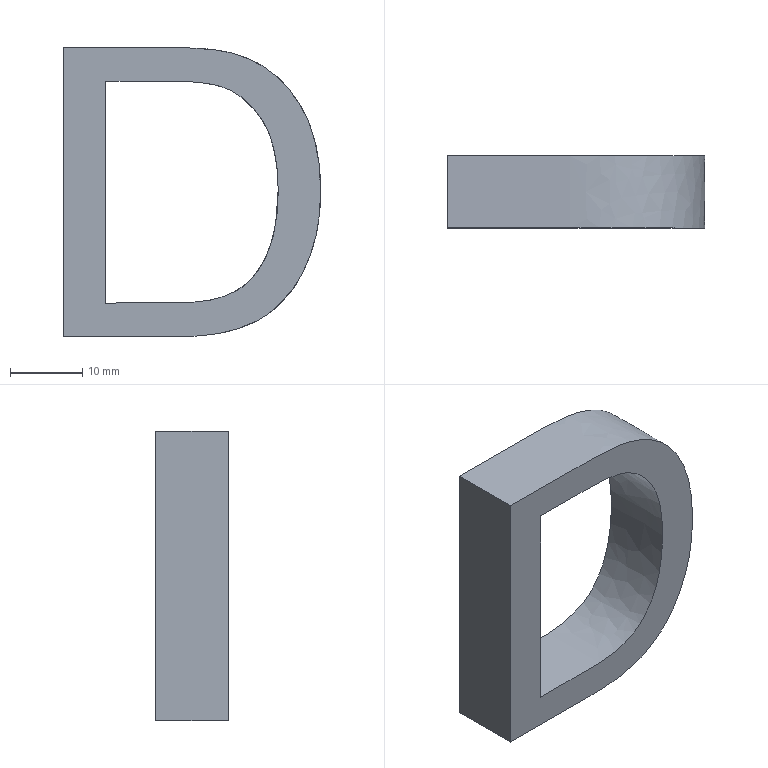Part | NX | features solid 2 | 1 solid | 7 faces | box 35.549 x 10 x 40 mm | volume 6202 mm3 | plane 5 | spline 2
STEP:
#1=CARTESIAN_POINT('',(-502.315,-915.,190.669));
#2=VERTEX_POINT('',#1);
#3=CARTESIAN_POINT('',(-502.315,-915.,159.985));
#4=VERTEX_POINT('',#3);
#5=CARTESIAN_POINT('',(-502.315,-915.,190.669));
#6=CARTESIAN_POINT('',(-502.315,-915.,180.441));
#7=CARTESIAN_POINT('',(-502.315,-915.,170.213));
#8=CARTESIAN_POINT('',(-502.315,-915.,159.985));
#9=B_SPLINE_CURVE_WITH_KNOTS('',3,(#5,#6,#7,#8),.UNSPECIFIED.,.F.,.F.,(4,4),(0.,0.305),.PIECEWISE_BEZIER_KNOTS.);
#10=EDGE_CURVE('',#2,#4,#9,.T.);
#11=ORIENTED_EDGE('',*,*,#10,.F.);
#12=CARTESIAN_POINT('',(-502.315,-925.,190.669));
#13=VERTEX_POINT('',#12);
#14=CARTESIAN_POINT('',(-502.315,-925.,190.669));
#15=DIRECTION('',(0.,1.,0.));
#16=VECTOR('',#15,1000.);
#17=LINE('',#14,#16);
#18=EDGE_CURVE('',#2,#13,#17,.F.);
#19=ORIENTED_EDGE('',*,*,#18,.T.);
#20=CARTESIAN_POINT('',(-502.315,-925.,159.985));
#21=VERTEX_POINT('',#20);
#22=CARTESIAN_POINT('',(-502.315,-925.,190.669));
#23=CARTESIAN_POINT('',(-502.315,-925.,180.441));
#24=CARTESIAN_POINT('',(-502.315,-925.,170.213));
#25=CARTESIAN_POINT('',(-502.315,-925.,159.985));
#26=B_SPLINE_CURVE_WITH_KNOTS('',3,(#22,#23,#24,#25),.UNSPECIFIED.,.F.,.F.,(4,4),(0.,0.305),.PIECEWISE_BEZIER_KNOTS.);
#27=EDGE_CURVE('',#13,#21,#26,.T.);
#28=ORIENTED_EDGE('',*,*,#27,.T.);
#29=CARTESIAN_POINT('',(-502.315,-925.,159.985));
#30=DIRECTION('',(0.,1.,0.));
#31=VECTOR('',#30,1000.);
#32=LINE('',#29,#31);
#33=EDGE_CURVE('',#21,#4,#32,.T.);
#34=ORIENTED_EDGE('',*,*,#33,.T.);
#35=EDGE_LOOP('',(#11,#19,#28,#34));
#36=FACE_BOUND('',#35,.T.);
#37=CARTESIAN_POINT('',(-502.315,-925.,190.669));
#38=DIRECTION('',(1.,0.,0.));
#39=DIRECTION('',(0.,1.,0.));
#40=AXIS2_PLACEMENT_3D('',#37,#38,#39);
#41=PLANE('',#40);
#42=ADVANCED_FACE('',(#36),#41,.T.);
#43=CARTESIAN_POINT('',(-492.679,-915.,155.335));
#44=VERTEX_POINT('',#43);
#45=CARTESIAN_POINT('',(-508.174,-915.,155.335));
#46=VERTEX_POINT('',#45);
#47=CARTESIAN_POINT('',(-492.679,-915.,155.335));
#48=CARTESIAN_POINT('',(-497.844,-915.,155.335));
#49=CARTESIAN_POINT('',(-503.009,-915.,155.335));
#50=CARTESIAN_POINT('',(-508.174,-915.,155.335));
#51=B_SPLINE_CURVE_WITH_KNOTS('',3,(#47,#48,#49,#50),.UNSPECIFIED.,.F.,.F.,(4,4),(0.,0.1123),.PIECEWISE_BEZIER_KNOTS.);
#52=EDGE_CURVE('',#44,#46,#51,.T.);
#53=ORIENTED_EDGE('',*,*,#52,.F.);
#54=CARTESIAN_POINT('',(-492.679,-925.,155.335));
#55=VERTEX_POINT('',#54);
#56=CARTESIAN_POINT('',(-492.679,-925.,155.335));
#57=DIRECTION('',(0.,1.,0.));
#58=VECTOR('',#57,1000.);
#59=LINE('',#56,#58);
#60=EDGE_CURVE('',#55,#44,#59,.T.);
#61=ORIENTED_EDGE('',*,*,#60,.F.);
#62=CARTESIAN_POINT('',(-508.174,-925.,155.335));
#63=VERTEX_POINT('',#62);
#64=CARTESIAN_POINT('',(-492.679,-925.,155.335));
#65=CARTESIAN_POINT('',(-497.844,-925.,155.335));
#66=CARTESIAN_POINT('',(-503.009,-925.,155.335));
#67=CARTESIAN_POINT('',(-508.174,-925.,155.335));
#68=B_SPLINE_CURVE_WITH_KNOTS('',3,(#64,#65,#66,#67),.UNSPECIFIED.,.F.,.F.,(4,4),(0.,0.1123),.PIECEWISE_BEZIER_KNOTS.);
#69=EDGE_CURVE('',#55,#63,#68,.T.);
#70=ORIENTED_EDGE('',*,*,#69,.T.);
#71=CARTESIAN_POINT('',(-508.174,-925.,155.335));
#72=DIRECTION('',(0.,1.,0.));
#73=VECTOR('',#72,1000.);
#74=LINE('',#71,#73);
#75=EDGE_CURVE('',#63,#46,#74,.T.);
#76=ORIENTED_EDGE('',*,*,#75,.T.);
#77=EDGE_LOOP('',(#53,#61,#70,#76));
#78=FACE_BOUND('',#77,.T.);
#79=CARTESIAN_POINT('',(-492.679,-925.,155.335));
#80=DIRECTION('',(0.,0.,-1.));
#81=DIRECTION('',(1.,0.,0.));
#82=AXIS2_PLACEMENT_3D('',#79,#80,#81);
#83=PLANE('',#82);
#84=ADVANCED_FACE('',(#78),#83,.T.);
#85=CARTESIAN_POINT('',(-508.174,-915.,195.335));
#86=VERTEX_POINT('',#85);
#87=CARTESIAN_POINT('',(-508.174,-915.,155.335));
#88=CARTESIAN_POINT('',(-508.174,-915.,168.668));
#89=CARTESIAN_POINT('',(-508.174,-915.,182.001));
#90=CARTESIAN_POINT('',(-508.174,-915.,195.335));
#91=B_SPLINE_CURVE_WITH_KNOTS('',3,(#87,#88,#89,#90),.UNSPECIFIED.,.F.,.F.,(4,4),(0.1123,0.4022),.PIECEWISE_BEZIER_KNOTS.);
#92=EDGE_CURVE('',#46,#86,#91,.T.);
#93=ORIENTED_EDGE('',*,*,#92,.F.);
#94=ORIENTED_EDGE('',*,*,#75,.F.);
#95=CARTESIAN_POINT('',(-508.174,-925.,195.335));
#96=VERTEX_POINT('',#95);
#97=CARTESIAN_POINT('',(-508.174,-925.,155.335));
#98=CARTESIAN_POINT('',(-508.174,-925.,168.668));
#99=CARTESIAN_POINT('',(-508.174,-925.,182.001));
#100=CARTESIAN_POINT('',(-508.174,-925.,195.335));
#101=B_SPLINE_CURVE_WITH_KNOTS('',3,(#97,#98,#99,#100),.UNSPECIFIED.,.F.,.F.,(4,4),(0.1123,0.4022),.PIECEWISE_BEZIER_KNOTS.);
#102=EDGE_CURVE('',#63,#96,#101,.T.);
#103=ORIENTED_EDGE('',*,*,#102,.T.);
#104=CARTESIAN_POINT('',(-508.174,-925.,195.335));
#105=DIRECTION('',(0.,1.,0.));
#106=VECTOR('',#105,1000.);
#107=LINE('',#104,#106);
#108=EDGE_CURVE('',#96,#86,#107,.T.);
#109=ORIENTED_EDGE('',*,*,#108,.T.);
#110=EDGE_LOOP('',(#93,#94,#103,#109));
#111=FACE_BOUND('',#110,.T.);
#112=CARTESIAN_POINT('',(-508.174,-925.,155.335));
#113=DIRECTION('',(-1.,0.,0.));
#114=DIRECTION('',(0.,-1.,0.));
#115=AXIS2_PLACEMENT_3D('',#112,#113,#114);
#116=PLANE('',#115);
#117=ADVANCED_FACE('',(#111),#116,.T.);
#118=CARTESIAN_POINT('',(-508.174,-915.,195.335));
#119=CARTESIAN_POINT('',(-503.243,-915.,195.335));
#120=CARTESIAN_POINT('',(-498.313,-915.,195.335));
#121=CARTESIAN_POINT('',(-493.382,-915.,195.316));
#122=CARTESIAN_POINT('',(-490.033,-915.,195.304));
#123=CARTESIAN_POINT('',(-487.478,-915.,195.12));
#124=CARTESIAN_POINT('',(-485.723,-915.,194.734));
#125=CARTESIAN_POINT('',(-483.241,-915.,194.187));
#126=CARTESIAN_POINT('',(-481.145,-915.,193.239));
#127=CARTESIAN_POINT('',(-477.114,-915.,190.099));
#128=CARTESIAN_POINT('',(-475.424,-915.,187.809));
#129=CARTESIAN_POINT('',(-473.152,-915.,182.251));
#130=CARTESIAN_POINT('',(-472.625,-915.,179.09));
#131=CARTESIAN_POINT('',(-472.625,-915.,172.497));
#132=CARTESIAN_POINT('',(-472.992,-915.,169.774));
#133=CARTESIAN_POINT('',(-474.551,-915.,165.098));
#134=CARTESIAN_POINT('',(-475.501,-915.,163.151));
#135=CARTESIAN_POINT('',(-476.697,-915.,161.612));
#136=CARTESIAN_POINT('',(-477.902,-915.,160.061));
#137=CARTESIAN_POINT('',(-479.218,-915.,158.868));
#138=CARTESIAN_POINT('',(-480.618,-915.,157.985));
#139=CARTESIAN_POINT('',(-482.033,-915.,157.094));
#140=CARTESIAN_POINT('',(-483.761,-915.,156.421));
#141=CARTESIAN_POINT('',(-485.777,-915.,155.965));
#142=CARTESIAN_POINT('',(-487.753,-915.,155.518));
#143=CARTESIAN_POINT('',(-490.063,-915.,155.335));
#144=CARTESIAN_POINT('',(-492.679,-915.,155.335));
#145=B_SPLINE_CURVE_WITH_KNOTS('',3,(#118,#119,#120,#121,#122,#123,#124,#125,#126,#127,#128,#129,#130,#131,#132,#133,#134,#135,#136,#137,#138,#139,#140,#141,#142,#143,#144),.UNSPECIFIED.,.F.,.F.,(4,3,3,2,2,2,2,3,3,3,4),(0.4022,0.5094,0.5652,0.6158,0.6832,0.7511,0.8099,0.8685,0.908,0.9489,1.),.UNSPECIFIED.);
#146=EDGE_CURVE('',#86,#44,#145,.T.);
#147=ORIENTED_EDGE('',*,*,#146,.F.);
#148=ORIENTED_EDGE('',*,*,#108,.F.);
#149=CARTESIAN_POINT('',(-508.174,-925.,195.335));
#150=CARTESIAN_POINT('',(-503.243,-925.,195.335));
#151=CARTESIAN_POINT('',(-498.313,-925.,195.335));
#152=CARTESIAN_POINT('',(-493.382,-925.,195.316));
#153=CARTESIAN_POINT('',(-490.033,-925.,195.304));
#154=CARTESIAN_POINT('',(-487.478,-925.,195.12));
#155=CARTESIAN_POINT('',(-485.723,-925.,194.734));
#156=CARTESIAN_POINT('',(-483.241,-925.,194.187));
#157=CARTESIAN_POINT('',(-481.145,-925.,193.239));
#158=CARTESIAN_POINT('',(-477.114,-925.,190.099));
#159=CARTESIAN_POINT('',(-475.424,-925.,187.809));
#160=CARTESIAN_POINT('',(-473.152,-925.,182.251));
#161=CARTESIAN_POINT('',(-472.625,-925.,179.09));
#162=CARTESIAN_POINT('',(-472.625,-925.,172.497));
#163=CARTESIAN_POINT('',(-472.992,-925.,169.774));
#164=CARTESIAN_POINT('',(-474.551,-925.,165.098));
#165=CARTESIAN_POINT('',(-475.501,-925.,163.151));
#166=CARTESIAN_POINT('',(-476.697,-925.,161.612));
#167=CARTESIAN_POINT('',(-477.902,-925.,160.061));
#168=CARTESIAN_POINT('',(-479.218,-925.,158.868));
#169=CARTESIAN_POINT('',(-480.618,-925.,157.985));
#170=CARTESIAN_POINT('',(-482.033,-925.,157.094));
#171=CARTESIAN_POINT('',(-483.761,-925.,156.421));
#172=CARTESIAN_POINT('',(-485.777,-925.,155.965));
#173=CARTESIAN_POINT('',(-487.753,-925.,155.518));
#174=CARTESIAN_POINT('',(-490.063,-925.,155.335));
#175=CARTESIAN_POINT('',(-492.679,-925.,155.335));
#176=B_SPLINE_CURVE_WITH_KNOTS('',3,(#149,#150,#151,#152,#153,#154,#155,#156,#157,#158,#159,#160,#161,#162,#163,#164,#165,#166,#167,#168,#169,#170,#171,#172,#173,#174,#175),.UNSPECIFIED.,.F.,.F.,(4,3,3,2,2,2,2,3,3,3,4),(0.4022,0.5094,0.5652,0.6158,0.6832,0.7511,0.8099,0.8685,0.908,0.9489,1.),.UNSPECIFIED.);
#177=EDGE_CURVE('',#96,#55,#176,.T.);
#178=ORIENTED_EDGE('',*,*,#177,.T.);
#179=ORIENTED_EDGE('',*,*,#60,.T.);
#180=EDGE_LOOP('',(#147,#148,#178,#179));
#181=FACE_BOUND('',#180,.T.);
#182=CARTESIAN_POINT('',(-508.174,-925.,195.335));
#183=CARTESIAN_POINT('',(-508.174,-915.,195.335));
#184=CARTESIAN_POINT('',(-506.456,-925.,195.335));
#185=CARTESIAN_POINT('',(-506.456,-915.,195.335));
#186=CARTESIAN_POINT('',(-503.024,-925.,195.335));
#187=CARTESIAN_POINT('',(-503.024,-915.,195.335));
#188=CARTESIAN_POINT('',(-498.712,-925.,195.331));
#189=CARTESIAN_POINT('',(-498.712,-915.,195.331));
#190=CARTESIAN_POINT('',(-495.733,-925.,195.324));
#191=CARTESIAN_POINT('',(-495.733,-915.,195.324));
#192=CARTESIAN_POINT('',(-494.191,-925.,195.319));
#193=CARTESIAN_POINT('',(-494.191,-915.,195.319));
#194=CARTESIAN_POINT('',(-493.395,-925.,195.317));
#195=CARTESIAN_POINT('',(-493.395,-915.,195.317));
#196=CARTESIAN_POINT('',(-492.212,-925.,195.308));
#197=CARTESIAN_POINT('',(-492.212,-915.,195.308));
#198=CARTESIAN_POINT('',(-490.966,-925.,195.278));
#199=CARTESIAN_POINT('',(-490.966,-915.,195.278));
#200=CARTESIAN_POINT('',(-489.064,-925.,195.189));
#201=CARTESIAN_POINT('',(-489.064,-915.,195.189));
#202=CARTESIAN_POINT('',(-487.474,-925.,195.043));
#203=CARTESIAN_POINT('',(-487.474,-915.,195.043));
#204=CARTESIAN_POINT('',(-486.259,-925.,194.845));
#205=CARTESIAN_POINT('',(-486.259,-915.,194.845));
#206=CARTESIAN_POINT('',(-485.712,-925.,194.735));
#207=CARTESIAN_POINT('',(-485.712,-915.,194.735));
#208=CARTESIAN_POINT('',(-484.717,-925.,194.497));
#209=CARTESIAN_POINT('',(-484.717,-915.,194.497));
#210=CARTESIAN_POINT('',(-483.685,-925.,194.182));
#211=CARTESIAN_POINT('',(-483.685,-915.,194.182));
#212=CARTESIAN_POINT('',(-482.048,-925.,193.55));
#213=CARTESIAN_POINT('',(-482.048,-915.,193.55));
#214=CARTESIAN_POINT('',(-480.225,-925.,192.563));
#215=CARTESIAN_POINT('',(-480.225,-915.,192.563));
#216=CARTESIAN_POINT('',(-477.696,-925.,190.54));
#217=CARTESIAN_POINT('',(-477.696,-915.,190.54));
#218=CARTESIAN_POINT('',(-475.237,-925.,187.471));
#219=CARTESIAN_POINT('',(-475.237,-915.,187.471));
#220=CARTESIAN_POINT('',(-473.335,-925.,182.853));
#221=CARTESIAN_POINT('',(-473.335,-915.,182.853));
#222=CARTESIAN_POINT('',(-472.652,-925.,178.499));
#223=CARTESIAN_POINT('',(-472.652,-915.,178.499));
#224=CARTESIAN_POINT('',(-472.599,-925.,174.588));
#225=CARTESIAN_POINT('',(-472.599,-915.,174.588));
#226=CARTESIAN_POINT('',(-472.786,-925.,171.836));
#227=CARTESIAN_POINT('',(-472.786,-915.,171.836));
#228=CARTESIAN_POINT('',(-473.2,-925.,169.307));
#229=CARTESIAN_POINT('',(-473.2,-915.,169.307));
#230=CARTESIAN_POINT('',(-473.884,-925.,167.));
#231=CARTESIAN_POINT('',(-473.884,-915.,167.));
#232=CARTESIAN_POINT('',(-474.706,-925.,164.93));
#233=CARTESIAN_POINT('',(-474.706,-915.,164.93));
#234=CARTESIAN_POINT('',(-475.487,-925.,163.404));
#235=CARTESIAN_POINT('',(-475.487,-915.,163.404));
#236=CARTESIAN_POINT('',(-476.09,-925.,162.447));
#237=CARTESIAN_POINT('',(-476.09,-915.,162.447));
#238=CARTESIAN_POINT('',(-476.459,-925.,161.924));
#239=CARTESIAN_POINT('',(-476.459,-915.,161.924));
#240=CARTESIAN_POINT('',(-476.727,-925.,161.568));
#241=CARTESIAN_POINT('',(-476.727,-915.,161.568));
#242=CARTESIAN_POINT('',(-477.203,-925.,160.982));
#243=CARTESIAN_POINT('',(-477.203,-915.,160.982));
#244=CARTESIAN_POINT('',(-477.78,-925.,160.331));
#245=CARTESIAN_POINT('',(-477.78,-915.,160.331));
#246=CARTESIAN_POINT('',(-478.852,-925.,159.252));
#247=CARTESIAN_POINT('',(-478.852,-915.,159.252));
#248=CARTESIAN_POINT('',(-480.447,-925.,158.012));
#249=CARTESIAN_POINT('',(-480.447,-915.,158.012));
#250=CARTESIAN_POINT('',(-482.153,-925.,157.115));
#251=CARTESIAN_POINT('',(-482.153,-915.,157.115));
#252=CARTESIAN_POINT('',(-483.761,-925.,156.509));
#253=CARTESIAN_POINT('',(-483.761,-915.,156.509));
#254=CARTESIAN_POINT('',(-484.804,-925.,156.198));
#255=CARTESIAN_POINT('',(-484.804,-915.,156.198));
#256=CARTESIAN_POINT('',(-485.767,-925.,155.964));
#257=CARTESIAN_POINT('',(-485.767,-915.,155.964));
#258=CARTESIAN_POINT('',(-486.456,-925.,155.819));
#259=CARTESIAN_POINT('',(-486.456,-915.,155.819));
#260=CARTESIAN_POINT('',(-487.823,-925.,155.585));
#261=CARTESIAN_POINT('',(-487.823,-915.,155.585));
#262=CARTESIAN_POINT('',(-489.886,-925.,155.385));
#263=CARTESIAN_POINT('',(-489.886,-915.,155.385));
#264=CARTESIAN_POINT('',(-491.722,-925.,155.335));
#265=CARTESIAN_POINT('',(-491.722,-915.,155.335));
#266=CARTESIAN_POINT('',(-492.679,-925.,155.335));
#267=CARTESIAN_POINT('',(-492.679,-915.,155.335));
#268=B_SPLINE_SURFACE_WITH_KNOTS('',3,1,((#182,#183),(#184,#185),(#186,#187),(#188,#189),(#190,#191),(#192,#193),(#194,#195),(#196,#197),(#198,#199),(#200,#201),(#202,#203),(#204,#205),(#206,#207),(#208,#209),(#210,#211),(#212,#213),(#214,#215),(#216,#217),(#218,#219),(#220,#221),(#222,#223),(#224,#225),(#226,#227),(#228,#229),(#230,#231),(#232,#233),(#234,#235),(#236,#237),(#238,#239),(#240,#241),(#242,#243),(#244,#245),(#246,#247),(#248,#249),(#250,#251),(#252,#253),(#254,#255),(#256,#257),(#258,#259),(#260,#261),(#262,#263),(#264,#265),(#266,#267)),.SURF_OF_LINEAR_EXTRUSION.,.F.,.F.,.F.,(4,1,1,1,1,1,1,1,1,1,1,1,1,1,1,1,1,1,1,1,1,1,1,1,1,1,1,1,1,1,1,1,1,1,1,1,1,1,1,1,4),(2,2),(0.4022,0.4396,0.477,0.4956,0.505,0.5096,0.5143,0.5237,0.533,0.5517,0.561,0.5657,0.5704,0.5797,0.589,0.6077,0.6264,0.6638,0.7011,0.7385,0.7572,0.7758,0.7945,0.8132,0.8319,0.8506,0.8599,0.8646,0.8692,0.8739,0.8786,0.8879,0.9066,0.9253,0.9346,0.944,0.9486,0.9533,0.9626,0.9813,1.),(0.,1.),.UNSPECIFIED.);
#269=ADVANCED_FACE('',(#181),#268,.T.);
#270=CARTESIAN_POINT('',(-502.315,-915.,159.985));
#271=CARTESIAN_POINT('',(-499.277,-915.,159.985));
#272=CARTESIAN_POINT('',(-496.238,-915.,159.985));
#273=CARTESIAN_POINT('',(-490.369,-915.,159.985));
#274=CARTESIAN_POINT('',(-488.182,-915.,160.214));
#275=CARTESIAN_POINT('',(-486.587,-915.,160.708));
#276=CARTESIAN_POINT('',(-484.969,-915.,161.208));
#277=CARTESIAN_POINT('',(-483.685,-915.,161.881));
#278=CARTESIAN_POINT('',(-482.72,-915.,162.782));
#279=CARTESIAN_POINT('',(-481.375,-915.,164.038));
#280=CARTESIAN_POINT('',(-480.335,-915.,165.736));
#281=CARTESIAN_POINT('',(-479.589,-915.,167.874));
#282=CARTESIAN_POINT('',(-478.851,-915.,169.989));
#283=CARTESIAN_POINT('',(-478.484,-915.,172.558));
#284=CARTESIAN_POINT('',(-478.484,-915.,179.793));
#285=CARTESIAN_POINT('',(-479.218,-915.,183.021));
#286=CARTESIAN_POINT('',(-480.683,-915.,185.277));
#287=CARTESIAN_POINT('',(-482.14,-915.,187.518));
#288=CARTESIAN_POINT('',(-483.945,-915.,189.048));
#289=CARTESIAN_POINT('',(-486.048,-915.,189.823));
#290=CARTESIAN_POINT('',(-487.554,-915.,190.379));
#291=CARTESIAN_POINT('',(-489.987,-915.,190.654));
#292=CARTESIAN_POINT('',(-496.34,-915.,190.683));
#293=CARTESIAN_POINT('',(-499.328,-915.,190.669));
#294=CARTESIAN_POINT('',(-502.315,-915.,190.669));
#295=B_SPLINE_CURVE_WITH_KNOTS('',3,(#270,#271,#272,#273,#274,#275,#276,#277,#278,#279,#280,#281,#282,#283,#284,#285,#286,#287,#288,#289,#290,#291,#292,#293,#294),.UNSPECIFIED.,.F.,.F.,(4,2,3,3,3,2,3,3,2,4),(0.305,0.3957,0.4801,0.5257,0.588,0.6692,0.78,0.8546,0.9316,1.),.UNSPECIFIED.);
#296=EDGE_CURVE('',#4,#2,#295,.T.);
#297=ORIENTED_EDGE('',*,*,#296,.F.);
#298=ORIENTED_EDGE('',*,*,#33,.F.);
#299=CARTESIAN_POINT('',(-502.315,-925.,159.985));
#300=CARTESIAN_POINT('',(-499.277,-925.,159.985));
#301=CARTESIAN_POINT('',(-496.238,-925.,159.985));
#302=CARTESIAN_POINT('',(-490.369,-925.,159.985));
#303=CARTESIAN_POINT('',(-488.182,-925.,160.214));
#304=CARTESIAN_POINT('',(-486.587,-925.,160.708));
#305=CARTESIAN_POINT('',(-484.969,-925.,161.208));
#306=CARTESIAN_POINT('',(-483.685,-925.,161.881));
#307=CARTESIAN_POINT('',(-482.72,-925.,162.782));
#308=CARTESIAN_POINT('',(-481.375,-925.,164.038));
#309=CARTESIAN_POINT('',(-480.335,-925.,165.736));
#310=CARTESIAN_POINT('',(-479.589,-925.,167.874));
#311=CARTESIAN_POINT('',(-478.851,-925.,169.989));
#312=CARTESIAN_POINT('',(-478.484,-925.,172.558));
#313=CARTESIAN_POINT('',(-478.484,-925.,179.793));
#314=CARTESIAN_POINT('',(-479.218,-925.,183.021));
#315=CARTESIAN_POINT('',(-480.683,-925.,185.277));
#316=CARTESIAN_POINT('',(-482.14,-925.,187.518));
#317=CARTESIAN_POINT('',(-483.945,-925.,189.048));
#318=CARTESIAN_POINT('',(-486.048,-925.,189.823));
#319=CARTESIAN_POINT('',(-487.554,-925.,190.379));
#320=CARTESIAN_POINT('',(-489.987,-925.,190.654));
#321=CARTESIAN_POINT('',(-496.34,-925.,190.683));
#322=CARTESIAN_POINT('',(-499.328,-925.,190.669));
#323=CARTESIAN_POINT('',(-502.315,-925.,190.669));
#324=B_SPLINE_CURVE_WITH_KNOTS('',3,(#299,#300,#301,#302,#303,#304,#305,#306,#307,#308,#309,#310,#311,#312,#313,#314,#315,#316,#317,#318,#319,#320,#321,#322,#323),.UNSPECIFIED.,.F.,.F.,(4,2,3,3,3,2,3,3,2,4),(0.305,0.3957,0.4801,0.5257,0.588,0.6692,0.78,0.8546,0.9316,1.),.UNSPECIFIED.);
#325=EDGE_CURVE('',#21,#13,#324,.T.);
#326=ORIENTED_EDGE('',*,*,#325,.T.);
#327=ORIENTED_EDGE('',*,*,#18,.F.);
#328=EDGE_LOOP('',(#297,#298,#326,#327));
#329=FACE_BOUND('',#328,.T.);
#330=CARTESIAN_POINT('',(-502.315,-925.,159.985));
#331=CARTESIAN_POINT('',(-502.315,-915.,159.985));
#332=CARTESIAN_POINT('',(-500.859,-925.,159.985));
#333=CARTESIAN_POINT('',(-500.859,-915.,159.985));
#334=CARTESIAN_POINT('',(-497.954,-925.,159.987));
#335=CARTESIAN_POINT('',(-497.954,-915.,159.987));
#336=CARTESIAN_POINT('',(-494.284,-925.,159.977));
#337=CARTESIAN_POINT('',(-494.284,-915.,159.977));
#338=CARTESIAN_POINT('',(-491.428,-925.,159.998));
#339=CARTESIAN_POINT('',(-491.428,-915.,159.998));
#340=CARTESIAN_POINT('',(-489.591,-925.,160.125));
#341=CARTESIAN_POINT('',(-489.591,-915.,160.125));
#342=CARTESIAN_POINT('',(-488.246,-925.,160.31));
#343=CARTESIAN_POINT('',(-488.246,-915.,160.31));
#344=CARTESIAN_POINT('',(-487.427,-925.,160.48));
#345=CARTESIAN_POINT('',(-487.427,-915.,160.48));
#346=CARTESIAN_POINT('',(-486.965,-925.,160.597));
#347=CARTESIAN_POINT('',(-486.965,-915.,160.597));
#348=CARTESIAN_POINT('',(-486.744,-925.,160.659));
#349=CARTESIAN_POINT('',(-486.744,-915.,160.659));
#350=CARTESIAN_POINT('',(-486.448,-925.,160.75));
#351=CARTESIAN_POINT('',(-486.448,-915.,160.75));
#352=CARTESIAN_POINT('',(-486.052,-925.,160.881));
#353=CARTESIAN_POINT('',(-486.052,-915.,160.881));
#354=CARTESIAN_POINT('',(-485.434,-925.,161.107));
#355=CARTESIAN_POINT('',(-485.434,-915.,161.107));
#356=CARTESIAN_POINT('',(-484.257,-925.,161.627));
#357=CARTESIAN_POINT('',(-484.257,-915.,161.627));
#358=CARTESIAN_POINT('',(-482.893,-925.,162.52));
#359=CARTESIAN_POINT('',(-482.893,-915.,162.52));
#360=CARTESIAN_POINT('',(-481.589,-925.,163.939));
#361=CARTESIAN_POINT('',(-481.589,-915.,163.939));
#362=CARTESIAN_POINT('',(-480.652,-925.,165.407));
#363=CARTESIAN_POINT('',(-480.652,-915.,165.407));
#364=CARTESIAN_POINT('',(-480.031,-925.,166.699));
#365=CARTESIAN_POINT('',(-480.031,-915.,166.699));
#366=CARTESIAN_POINT('',(-479.58,-925.,167.865));
#367=CARTESIAN_POINT('',(-479.58,-915.,167.865));
#368=CARTESIAN_POINT('',(-479.327,-925.,168.67));
#369=CARTESIAN_POINT('',(-479.327,-915.,168.67));
#370=CARTESIAN_POINT('',(-479.,-925.,169.917));
#371=CARTESIAN_POINT('',(-479.,-915.,169.917));
#372=CARTESIAN_POINT('',(-478.705,-925.,171.568));
#373=CARTESIAN_POINT('',(-478.705,-915.,171.568));
#374=CARTESIAN_POINT('',(-478.504,-925.,173.746));
#375=CARTESIAN_POINT('',(-478.504,-915.,173.746));
#376=CARTESIAN_POINT('',(-478.46,-925.,176.206));
#377=CARTESIAN_POINT('',(-478.46,-915.,176.206));
#378=CARTESIAN_POINT('',(-478.584,-925.,178.517));
#379=CARTESIAN_POINT('',(-478.584,-915.,178.517));
#380=CARTESIAN_POINT('',(-478.877,-925.,180.589));
#381=CARTESIAN_POINT('',(-478.877,-915.,180.589));
#382=CARTESIAN_POINT('',(-479.338,-925.,182.443));
#383=CARTESIAN_POINT('',(-479.338,-915.,182.443));
#384=CARTESIAN_POINT('',(-479.868,-925.,183.809));
#385=CARTESIAN_POINT('',(-479.868,-915.,183.809));
#386=CARTESIAN_POINT('',(-480.302,-925.,184.653));
#387=CARTESIAN_POINT('',(-480.302,-915.,184.653));
#388=CARTESIAN_POINT('',(-480.552,-925.,185.071));
#389=CARTESIAN_POINT('',(-480.552,-915.,185.071));
#390=CARTESIAN_POINT('',(-480.678,-925.,185.269));
#391=CARTESIAN_POINT('',(-480.678,-915.,185.269));
#392=CARTESIAN_POINT('',(-481.027,-925.,185.797));
#393=CARTESIAN_POINT('',(-481.027,-915.,185.797));
#394=CARTESIAN_POINT('',(-481.507,-925.,186.444));
#395=CARTESIAN_POINT('',(-481.507,-915.,186.444));
#396=CARTESIAN_POINT('',(-482.466,-925.,187.55));
#397=CARTESIAN_POINT('',(-482.466,-915.,187.55));
#398=CARTESIAN_POINT('',(-483.492,-925.,188.448));
#399=CARTESIAN_POINT('',(-483.492,-915.,188.448));
#400=CARTESIAN_POINT('',(-484.616,-925.,189.171));
#401=CARTESIAN_POINT('',(-484.616,-915.,189.171));
#402=CARTESIAN_POINT('',(-485.324,-925.,189.534));
#403=CARTESIAN_POINT('',(-485.324,-915.,189.534));
#404=CARTESIAN_POINT('',(-485.97,-925.,189.798));
#405=CARTESIAN_POINT('',(-485.97,-915.,189.798));
#406=CARTESIAN_POINT('',(-486.407,-925.,189.951));
#407=CARTESIAN_POINT('',(-486.407,-915.,189.951));
#408=CARTESIAN_POINT('',(-487.264,-925.,190.191));
#409=CARTESIAN_POINT('',(-487.264,-915.,190.191));
#410=CARTESIAN_POINT('',(-488.771,-925.,190.45));
#411=CARTESIAN_POINT('',(-488.771,-915.,190.45));
#412=CARTESIAN_POINT('',(-491.,-925.,190.637));
#413=CARTESIAN_POINT('',(-491.,-915.,190.637));
#414=CARTESIAN_POINT('',(-493.753,-925.,190.678));
#415=CARTESIAN_POINT('',(-493.753,-915.,190.678));
#416=CARTESIAN_POINT('',(-497.581,-925.,190.675));
#417=CARTESIAN_POINT('',(-497.581,-915.,190.675));
#418=CARTESIAN_POINT('',(-500.417,-925.,190.669));
#419=CARTESIAN_POINT('',(-500.417,-915.,190.669));
#420=CARTESIAN_POINT('',(-502.315,-925.,190.669));
#421=CARTESIAN_POINT('',(-502.315,-915.,190.669));
#422=B_SPLINE_SURFACE_WITH_KNOTS('',3,1,((#330,#331),(#332,#333),(#334,#335),(#336,#337),(#338,#339),(#340,#341),(#342,#343),(#344,#345),(#346,#347),(#348,#349),(#350,#351),(#352,#353),(#354,#355),(#356,#357),(#358,#359),(#360,#361),(#362,#363),(#364,#365),(#366,#367),(#368,#369),(#370,#371),(#372,#373),(#374,#375),(#376,#377),(#378,#379),(#380,#381),(#382,#383),(#384,#385),(#386,#387),(#388,#389),(#390,#391),(#392,#393),(#394,#395),(#396,#397),(#398,#399),(#400,#401),(#402,#403),(#404,#405),(#406,#407),(#408,#409),(#410,#411),(#412,#413),(#414,#415),(#416,#417),(#418,#419),(#420,#421)),.SURF_OF_LINEAR_EXTRUSION.,.F.,.F.,.F.,(4,1,1,1,1,1,1,1,1,1,1,1,1,1,1,1,1,1,1,1,1,1,1,1,1,1,1,1,1,1,1,1,1,1,1,1,1,1,1,1,1,1,1,4),(2,2),(0.305,0.3485,0.3919,0.4136,0.4353,0.4571,0.4679,0.4733,0.4788,0.4815,0.4842,0.4896,0.5005,0.5222,0.5439,0.5656,0.5765,0.5874,0.5982,0.6091,0.6308,0.6525,0.6742,0.696,0.7177,0.7394,0.7611,0.772,0.7774,0.7801,0.7828,0.7937,0.8045,0.8263,0.8371,0.848,0.8534,0.8588,0.8697,0.8914,0.9131,0.9348,0.9566,1.),(0.,1.),.UNSPECIFIED.);
#423=ADVANCED_FACE('',(#329),#422,.T.);
#424=ORIENTED_EDGE('',*,*,#69,.F.);
#425=ORIENTED_EDGE('',*,*,#177,.F.);
#426=ORIENTED_EDGE('',*,*,#102,.F.);
#427=EDGE_LOOP('',(#424,#425,#426));
#428=FACE_BOUND('',#427,.T.);
#429=ORIENTED_EDGE('',*,*,#27,.F.);
#430=ORIENTED_EDGE('',*,*,#325,.F.);
#431=EDGE_LOOP('',(#429,#430));
#432=FACE_BOUND('',#431,.T.);
#433=CARTESIAN_POINT('',(-473.516,-925.,182.752));
#434=DIRECTION('',(0.,-1.,0.));
#435=DIRECTION('',(1.,0.,0.));
#436=AXIS2_PLACEMENT_3D('',#433,#434,#435);
#437=PLANE('',#436);
#438=ADVANCED_FACE('',(#428,#432),#437,.T.);
#439=ORIENTED_EDGE('',*,*,#52,.T.);
#440=ORIENTED_EDGE('',*,*,#92,.T.);
#441=ORIENTED_EDGE('',*,*,#146,.T.);
#442=EDGE_LOOP('',(#439,#440,#441));
#443=FACE_BOUND('',#442,.T.);
#444=ORIENTED_EDGE('',*,*,#10,.T.);
#445=ORIENTED_EDGE('',*,*,#296,.T.);
#446=EDGE_LOOP('',(#444,#445));
#447=FACE_BOUND('',#446,.T.);
#448=CARTESIAN_POINT('',(-473.516,-915.,182.752));
#449=DIRECTION('',(0.,-1.,0.));
#450=DIRECTION('',(1.,0.,0.));
#451=AXIS2_PLACEMENT_3D('',#448,#449,#450);
#452=PLANE('',#451);
#453=ADVANCED_FACE('',(#443,#447),#452,.F.);
#454=CLOSED_SHELL('',(#42,#84,#117,#269,#423,#438,#453));
#455=MANIFOLD_SOLID_BREP('',#454);
#456=(LENGTH_UNIT()NAMED_UNIT(*)SI_UNIT(.MILLI.,.METRE.));
#457=UNCERTAINTY_MEASURE_WITH_UNIT(LENGTH_MEASURE(0.0508),#456,'','');
#458=(NAMED_UNIT(*)PLANE_ANGLE_UNIT()SI_UNIT($,.RADIAN.));
#459=(NAMED_UNIT(*)SI_UNIT($,.STERADIAN.)SOLID_ANGLE_UNIT());
#460=(GEOMETRIC_REPRESENTATION_CONTEXT(3)GLOBAL_UNCERTAINTY_ASSIGNED_CONTEXT((#457))GLOBAL_UNIT_ASSIGNED_CONTEXT((#456,#458,#459))REPRESENTATION_CONTEXT('',''));
#461=ADVANCED_BREP_SHAPE_REPRESENTATION('',(#455),#460);